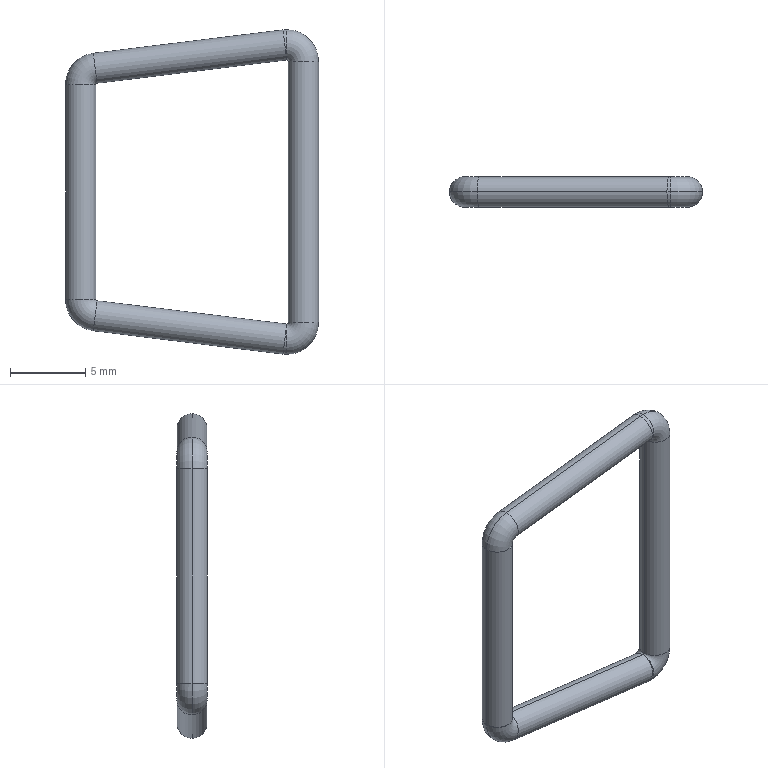Part | SolidWorks | features RefAxis 6, Revolution 4, ICE 3, 3DProfileFeature 2, Extrusion 1 | 1 solid | 24 faces | box 16.763 x 2 x 21.5 mm | volume 200.249 mm3 | torus 12 | cylinder 8 | plane 4 | commonest cylinder face diameters 2 x8
STEP:
#1=CARTESIAN_POINT('',(-7.193,0.,7.107));
#2=VERTEX_POINT('',#1);
#3=CARTESIAN_POINT('',(-6.185,1.,7.107));
#4=VERTEX_POINT('',#3);
#5=CARTESIAN_POINT('',(-6.193,0.,7.107));
#6=DIRECTION('',(0.,0.,-1.));
#7=DIRECTION('',(-1.,0.,0.));
#8=AXIS2_PLACEMENT_3D('',#5,#6,#7);
#9=CIRCLE('',#8,1.);
#10=EDGE_CURVE('',#2,#4,#9,.T.);
#11=ORIENTED_EDGE('',*,*,#10,.F.);
#12=CARTESIAN_POINT('',(-5.349,0.,9.192));
#13=VERTEX_POINT('',#12);
#14=CARTESIAN_POINT('',(-5.093,0.,7.107));
#15=DIRECTION('',(0.,1.,0.));
#16=DIRECTION('',(0.,0.,1.));
#17=AXIS2_PLACEMENT_3D('',#14,#15,#16);
#18=CIRCLE('',#17,2.1);
#19=EDGE_CURVE('',#2,#13,#18,.T.);
#20=ORIENTED_EDGE('',*,*,#19,.T.);
#21=CARTESIAN_POINT('',(-5.105,0.,7.207));
#22=VERTEX_POINT('',#21);
#23=CARTESIAN_POINT('',(-5.227,0.,8.199));
#24=DIRECTION('',(-0.9925,0.,-0.1219));
#25=DIRECTION('',(-0.1219,0.,0.9925));
#26=AXIS2_PLACEMENT_3D('',#23,#24,#25);
#27=CIRCLE('',#26,1.);
#28=EDGE_CURVE('',#13,#22,#27,.T.);
#29=ORIENTED_EDGE('',*,*,#28,.T.);
#30=CARTESIAN_POINT('',(-5.193,0.,7.107));
#31=VERTEX_POINT('',#30);
#32=CARTESIAN_POINT('',(-5.093,0.,7.107));
#33=DIRECTION('',(0.,1.,0.));
#34=DIRECTION('',(0.,0.,1.));
#35=AXIS2_PLACEMENT_3D('',#32,#33,#34);
#36=CIRCLE('',#35,0.1);
#37=EDGE_CURVE('',#31,#22,#36,.T.);
#38=ORIENTED_EDGE('',*,*,#37,.F.);
#39=CARTESIAN_POINT('',(-6.193,0.,7.107));
#40=DIRECTION('',(0.,0.,-1.));
#41=DIRECTION('',(-1.,0.,0.));
#42=AXIS2_PLACEMENT_3D('',#39,#40,#41);
#43=CIRCLE('',#42,1.);
#44=EDGE_CURVE('',#4,#31,#43,.T.);
#45=ORIENTED_EDGE('',*,*,#44,.F.);
#46=EDGE_LOOP('',(#11,#20,#29,#38,#45));
#47=FACE_OUTER_BOUND('',#46,.T.);
#48=CARTESIAN_POINT('',(-5.093,0.,7.107));
#49=DIRECTION('',(0.,1.,0.));
#50=DIRECTION('',(0.,0.,1.));
#51=AXIS2_PLACEMENT_3D('',#48,#49,#50);
#52=TOROIDAL_SURFACE('',#51,1.1,1.);
#53=ADVANCED_FACE('',(#47),#52,.T.);
#54=CARTESIAN_POINT('',(-7.193,0.,-7.107));
#55=VERTEX_POINT('',#54);
#56=CARTESIAN_POINT('',(-6.185,-1.,-7.107));
#57=VERTEX_POINT('',#56);
#58=CARTESIAN_POINT('',(-6.193,0.,-7.107));
#59=DIRECTION('',(0.,0.,1.));
#60=DIRECTION('',(1.,0.,0.));
#61=AXIS2_PLACEMENT_3D('',#58,#59,#60);
#62=CIRCLE('',#61,1.);
#63=EDGE_CURVE('',#55,#57,#62,.T.);
#64=ORIENTED_EDGE('',*,*,#63,.F.);
#65=CARTESIAN_POINT('',(-5.349,0.,-9.192));
#66=VERTEX_POINT('',#65);
#67=CARTESIAN_POINT('',(-5.093,0.,-7.107));
#68=DIRECTION('',(0.,-1.,0.));
#69=DIRECTION('',(0.,0.,-1.));
#70=AXIS2_PLACEMENT_3D('',#67,#68,#69);
#71=CIRCLE('',#70,2.1);
#72=EDGE_CURVE('',#55,#66,#71,.T.);
#73=ORIENTED_EDGE('',*,*,#72,.T.);
#74=CARTESIAN_POINT('',(-5.105,0.,-7.207));
#75=VERTEX_POINT('',#74);
#76=CARTESIAN_POINT('',(-5.227,0.,-8.199));
#77=DIRECTION('',(-0.9925,0.,0.1219));
#78=DIRECTION('',(0.1219,0.,0.9925));
#79=AXIS2_PLACEMENT_3D('',#76,#77,#78);
#80=CIRCLE('',#79,1.);
#81=EDGE_CURVE('',#66,#75,#80,.T.);
#82=ORIENTED_EDGE('',*,*,#81,.T.);
#83=CARTESIAN_POINT('',(-5.193,0.,-7.107));
#84=VERTEX_POINT('',#83);
#85=CARTESIAN_POINT('',(-5.093,0.,-7.107));
#86=DIRECTION('',(0.,-1.,0.));
#87=DIRECTION('',(0.,0.,-1.));
#88=AXIS2_PLACEMENT_3D('',#85,#86,#87);
#89=CIRCLE('',#88,0.1);
#90=EDGE_CURVE('',#84,#75,#89,.T.);
#91=ORIENTED_EDGE('',*,*,#90,.F.);
#92=CARTESIAN_POINT('',(-6.193,0.,-7.107));
#93=DIRECTION('',(0.,0.,1.));
#94=DIRECTION('',(1.,0.,0.));
#95=AXIS2_PLACEMENT_3D('',#92,#93,#94);
#96=CIRCLE('',#95,1.);
#97=EDGE_CURVE('',#57,#84,#96,.T.);
#98=ORIENTED_EDGE('',*,*,#97,.F.);
#99=EDGE_LOOP('',(#64,#73,#82,#91,#98));
#100=FACE_OUTER_BOUND('',#99,.T.);
#101=CARTESIAN_POINT('',(-5.093,0.,-7.107));
#102=DIRECTION('',(0.,-1.,0.));
#103=DIRECTION('',(0.,0.,-1.));
#104=AXIS2_PLACEMENT_3D('',#101,#102,#103);
#105=TOROIDAL_SURFACE('',#104,1.1,1.);
#106=ADVANCED_FACE('',(#100),#105,.T.);
#107=CARTESIAN_POINT('',(7.47,0.,10.75));
#108=VERTEX_POINT('',#107);
#109=CARTESIAN_POINT('',(7.47,0.,8.75));
#110=VERTEX_POINT('',#109);
#111=CARTESIAN_POINT('',(7.47,0.,9.75));
#112=DIRECTION('',(-1.,0.,0.));
#113=DIRECTION('',(0.,0.,1.));
#114=AXIS2_PLACEMENT_3D('',#111,#112,#113);
#115=CIRCLE('',#114,1.);
#116=EDGE_CURVE('',#108,#110,#115,.T.);
#117=ORIENTED_EDGE('',*,*,#116,.F.);
#118=CARTESIAN_POINT('',(9.57,0.,8.65));
#119=VERTEX_POINT('',#118);
#120=CARTESIAN_POINT('',(7.47,0.,8.65));
#121=DIRECTION('',(0.,1.,0.));
#122=DIRECTION('',(0.,0.,1.));
#123=AXIS2_PLACEMENT_3D('',#120,#121,#122);
#124=CIRCLE('',#123,2.1);
#125=EDGE_CURVE('',#108,#119,#124,.T.);
#126=ORIENTED_EDGE('',*,*,#125,.T.);
#127=CARTESIAN_POINT('',(7.57,0.,8.65));
#128=VERTEX_POINT('',#127);
#129=CARTESIAN_POINT('',(8.57,0.,8.65));
#130=DIRECTION('',(0.,0.,1.));
#131=DIRECTION('',(1.,0.,0.));
#132=AXIS2_PLACEMENT_3D('',#129,#130,#131);
#133=CIRCLE('',#132,1.);
#134=EDGE_CURVE('',#119,#128,#133,.T.);
#135=ORIENTED_EDGE('',*,*,#134,.T.);
#136=CARTESIAN_POINT('',(7.47,0.,8.65));
#137=DIRECTION('',(0.,1.,0.));
#138=DIRECTION('',(0.,0.,1.));
#139=AXIS2_PLACEMENT_3D('',#136,#137,#138);
#140=CIRCLE('',#139,0.1);
#141=EDGE_CURVE('',#110,#128,#140,.T.);
#142=ORIENTED_EDGE('',*,*,#141,.F.);
#143=EDGE_LOOP('',(#117,#126,#135,#142));
#144=FACE_OUTER_BOUND('',#143,.T.);
#145=CARTESIAN_POINT('',(7.47,0.,8.65));
#146=DIRECTION('',(0.,1.,0.));
#147=DIRECTION('',(0.,0.,1.));
#148=AXIS2_PLACEMENT_3D('',#145,#146,#147);
#149=TOROIDAL_SURFACE('',#148,1.1,1.);
#150=ADVANCED_FACE('',(#144),#149,.T.);
#151=CARTESIAN_POINT('',(7.47,0.,-10.75));
#152=VERTEX_POINT('',#151);
#153=CARTESIAN_POINT('',(7.47,0.,-8.75));
#154=VERTEX_POINT('',#153);
#155=CARTESIAN_POINT('',(7.47,0.,-9.75));
#156=DIRECTION('',(-1.,0.,0.));
#157=DIRECTION('',(0.,0.,1.));
#158=AXIS2_PLACEMENT_3D('',#155,#156,#157);
#159=CIRCLE('',#158,1.);
#160=EDGE_CURVE('',#152,#154,#159,.T.);
#161=ORIENTED_EDGE('',*,*,#160,.F.);
#162=CARTESIAN_POINT('',(9.57,0.,-8.65));
#163=VERTEX_POINT('',#162);
#164=CARTESIAN_POINT('',(7.47,0.,-8.65));
#165=DIRECTION('',(0.,-1.,0.));
#166=DIRECTION('',(0.,0.,-1.));
#167=AXIS2_PLACEMENT_3D('',#164,#165,#166);
#168=CIRCLE('',#167,2.1);
#169=EDGE_CURVE('',#152,#163,#168,.T.);
#170=ORIENTED_EDGE('',*,*,#169,.T.);
#171=CARTESIAN_POINT('',(7.57,0.,-8.65));
#172=VERTEX_POINT('',#171);
#173=CARTESIAN_POINT('',(8.57,0.,-8.65));
#174=DIRECTION('',(0.,0.,1.));
#175=DIRECTION('',(1.,0.,0.));
#176=AXIS2_PLACEMENT_3D('',#173,#174,#175);
#177=CIRCLE('',#176,1.);
#178=EDGE_CURVE('',#172,#163,#177,.T.);
#179=ORIENTED_EDGE('',*,*,#178,.F.);
#180=CARTESIAN_POINT('',(7.47,0.,-8.65));
#181=DIRECTION('',(0.,-1.,0.));
#182=DIRECTION('',(0.,0.,-1.));
#183=AXIS2_PLACEMENT_3D('',#180,#181,#182);
#184=CIRCLE('',#183,0.1);
#185=EDGE_CURVE('',#154,#172,#184,.T.);
#186=ORIENTED_EDGE('',*,*,#185,.F.);
#187=EDGE_LOOP('',(#161,#170,#179,#186));
#188=FACE_OUTER_BOUND('',#187,.T.);
#189=CARTESIAN_POINT('',(7.47,0.,-8.65));
#190=DIRECTION('',(0.,-1.,0.));
#191=DIRECTION('',(0.,0.,-1.));
#192=AXIS2_PLACEMENT_3D('',#189,#190,#191);
#193=TOROIDAL_SURFACE('',#192,1.1,1.);
#194=ADVANCED_FACE('',(#188),#193,.T.);
#195=CARTESIAN_POINT('',(7.214,0.,-10.734));
#196=VERTEX_POINT('',#195);
#197=CARTESIAN_POINT('',(7.458,0.,-8.749));
#198=VERTEX_POINT('',#197);
#199=CARTESIAN_POINT('',(7.336,0.,-9.742));
#200=DIRECTION('',(-0.9925,0.,0.1219));
#201=DIRECTION('',(0.1219,0.,0.9925));
#202=AXIS2_PLACEMENT_3D('',#199,#200,#201);
#203=CIRCLE('',#202,1.);
#204=EDGE_CURVE('',#196,#198,#203,.T.);
#205=ORIENTED_EDGE('',*,*,#204,.F.);
#206=CARTESIAN_POINT('',(7.47,0.,-8.65));
#207=DIRECTION('',(0.,-1.,0.));
#208=DIRECTION('',(0.,0.,-1.));
#209=AXIS2_PLACEMENT_3D('',#206,#207,#208);
#210=CIRCLE('',#209,2.1);
#211=EDGE_CURVE('',#196,#152,#210,.T.);
#212=ORIENTED_EDGE('',*,*,#211,.T.);
#213=ORIENTED_EDGE('',*,*,#160,.T.);
#214=CARTESIAN_POINT('',(7.47,0.,-8.65));
#215=DIRECTION('',(0.,-1.,0.));
#216=DIRECTION('',(0.,0.,-1.));
#217=AXIS2_PLACEMENT_3D('',#214,#215,#216);
#218=CIRCLE('',#217,0.1);
#219=EDGE_CURVE('',#198,#154,#218,.T.);
#220=ORIENTED_EDGE('',*,*,#219,.F.);
#221=EDGE_LOOP('',(#205,#212,#213,#220));
#222=FACE_OUTER_BOUND('',#221,.T.);
#223=CARTESIAN_POINT('',(7.47,0.,-8.65));
#224=DIRECTION('',(0.,-1.,0.));
#225=DIRECTION('',(0.,0.,-1.));
#226=AXIS2_PLACEMENT_3D('',#223,#224,#225);
#227=TOROIDAL_SURFACE('',#226,1.1,1.);
#228=ADVANCED_FACE('',(#222),#227,.T.);
#229=CARTESIAN_POINT('',(7.214,0.,10.734));
#230=VERTEX_POINT('',#229);
#231=CARTESIAN_POINT('',(7.458,0.,8.749));
#232=VERTEX_POINT('',#231);
#233=CARTESIAN_POINT('',(7.336,0.,9.742));
#234=DIRECTION('',(-0.9925,0.,-0.1219));
#235=DIRECTION('',(-0.1219,0.,0.9925));
#236=AXIS2_PLACEMENT_3D('',#233,#234,#235);
#237=CIRCLE('',#236,1.);
#238=EDGE_CURVE('',#230,#232,#237,.T.);
#239=ORIENTED_EDGE('',*,*,#238,.F.);
#240=CARTESIAN_POINT('',(7.47,0.,8.65));
#241=DIRECTION('',(0.,1.,0.));
#242=DIRECTION('',(0.,0.,1.));
#243=AXIS2_PLACEMENT_3D('',#240,#241,#242);
#244=CIRCLE('',#243,2.1);
#245=EDGE_CURVE('',#230,#108,#244,.T.);
#246=ORIENTED_EDGE('',*,*,#245,.T.);
#247=ORIENTED_EDGE('',*,*,#116,.T.);
#248=CARTESIAN_POINT('',(7.47,0.,8.65));
#249=DIRECTION('',(0.,1.,0.));
#250=DIRECTION('',(0.,0.,1.));
#251=AXIS2_PLACEMENT_3D('',#248,#249,#250);
#252=CIRCLE('',#251,0.1);
#253=EDGE_CURVE('',#232,#110,#252,.T.);
#254=ORIENTED_EDGE('',*,*,#253,.F.);
#255=EDGE_LOOP('',(#239,#246,#247,#254));
#256=FACE_OUTER_BOUND('',#255,.T.);
#257=CARTESIAN_POINT('',(7.47,0.,8.65));
#258=DIRECTION('',(0.,1.,0.));
#259=DIRECTION('',(0.,0.,1.));
#260=AXIS2_PLACEMENT_3D('',#257,#258,#259);
#261=TOROIDAL_SURFACE('',#260,1.1,1.);
#262=ADVANCED_FACE('',(#256),#261,.T.);
#263=CARTESIAN_POINT('',(-5.177,0.,7.107));
#264=VERTEX_POINT('',#263);
#265=CARTESIAN_POINT('',(-6.177,0.,7.107));
#266=DIRECTION('',(0.,0.,1.));
#267=DIRECTION('',(1.,0.,0.));
#268=AXIS2_PLACEMENT_3D('',#265,#266,#267);
#269=CIRCLE('',#268,1.);
#270=EDGE_CURVE('',#264,#4,#269,.T.);
#271=ORIENTED_EDGE('',*,*,#270,.F.);
#272=CARTESIAN_POINT('',(-5.177,0.,-7.107));
#273=VERTEX_POINT('',#272);
#274=CARTESIAN_POINT('',(-5.177,0.,7.107));
#275=DIRECTION('',(0.,0.,-1.));
#276=VECTOR('',#275,1000.);
#277=LINE('',#274,#276);
#278=EDGE_CURVE('',#264,#273,#277,.T.);
#279=ORIENTED_EDGE('',*,*,#278,.T.);
#280=CARTESIAN_POINT('',(-6.185,1.,-7.107));
#281=VERTEX_POINT('',#280);
#282=CARTESIAN_POINT('',(-6.177,0.,-7.107));
#283=DIRECTION('',(0.,0.,1.));
#284=DIRECTION('',(1.,0.,0.));
#285=AXIS2_PLACEMENT_3D('',#282,#283,#284);
#286=CIRCLE('',#285,1.);
#287=EDGE_CURVE('',#273,#281,#286,.T.);
#288=ORIENTED_EDGE('',*,*,#287,.T.);
#289=CARTESIAN_POINT('',(-7.177,0.,-7.107));
#290=VERTEX_POINT('',#289);
#291=CARTESIAN_POINT('',(-6.177,0.,-7.107));
#292=DIRECTION('',(0.,0.,1.));
#293=DIRECTION('',(1.,0.,0.));
#294=AXIS2_PLACEMENT_3D('',#291,#292,#293);
#295=CIRCLE('',#294,1.);
#296=EDGE_CURVE('',#281,#290,#295,.T.);
#297=ORIENTED_EDGE('',*,*,#296,.T.);
#298=CARTESIAN_POINT('',(-7.177,0.,7.107));
#299=VERTEX_POINT('',#298);
#300=CARTESIAN_POINT('',(-7.177,0.,7.107));
#301=DIRECTION('',(0.,0.,-1.));
#302=VECTOR('',#301,1000.);
#303=LINE('',#300,#302);
#304=EDGE_CURVE('',#299,#290,#303,.T.);
#305=ORIENTED_EDGE('',*,*,#304,.F.);
#306=CARTESIAN_POINT('',(-6.177,0.,7.107));
#307=DIRECTION('',(0.,0.,1.));
#308=DIRECTION('',(1.,0.,0.));
#309=AXIS2_PLACEMENT_3D('',#306,#307,#308);
#310=CIRCLE('',#309,1.);
#311=EDGE_CURVE('',#4,#299,#310,.T.);
#312=ORIENTED_EDGE('',*,*,#311,.F.);
#313=EDGE_LOOP('',(#271,#279,#288,#297,#305,#312));
#314=FACE_OUTER_BOUND('',#313,.T.);
#315=CARTESIAN_POINT('',(-6.177,0.,7.107));
#316=DIRECTION('',(0.,0.,-1.));
#317=DIRECTION('',(-1.,0.,0.));
#318=AXIS2_PLACEMENT_3D('',#315,#316,#317);
#319=CYLINDRICAL_SURFACE('',#318,1.);
#320=ADVANCED_FACE('',(#314),#319,.T.);
#321=ORIENTED_EDGE('',*,*,#28,.F.);
#322=CARTESIAN_POINT('',(-5.349,0.,9.192));
#323=DIRECTION('',(0.9925,0.,0.1219));
#324=VECTOR('',#323,1000.);
#325=LINE('',#322,#324);
#326=EDGE_CURVE('',#13,#230,#325,.T.);
#327=ORIENTED_EDGE('',*,*,#326,.T.);
#328=ORIENTED_EDGE('',*,*,#238,.T.);
#329=CARTESIAN_POINT('',(-5.105,0.,7.207));
#330=DIRECTION('',(0.9925,0.,0.1219));
#331=VECTOR('',#330,1000.);
#332=LINE('',#329,#331);
#333=EDGE_CURVE('',#22,#232,#332,.T.);
#334=ORIENTED_EDGE('',*,*,#333,.F.);
#335=EDGE_LOOP('',(#321,#327,#328,#334));
#336=FACE_OUTER_BOUND('',#335,.T.);
#337=CARTESIAN_POINT('',(-5.227,0.,8.199));
#338=DIRECTION('',(0.9925,0.,0.1219));
#339=DIRECTION('',(0.1219,0.,-0.9925));
#340=AXIS2_PLACEMENT_3D('',#337,#338,#339);
#341=CYLINDRICAL_SURFACE('',#340,1.);
#342=ADVANCED_FACE('',(#336),#341,.T.);
#343=CARTESIAN_POINT('',(-5.227,0.,-8.199));
#344=DIRECTION('',(-0.9925,0.,0.1219));
#345=DIRECTION('',(0.1219,0.,0.9925));
#346=AXIS2_PLACEMENT_3D('',#343,#344,#345);
#347=CIRCLE('',#346,1.);
#348=EDGE_CURVE('',#75,#66,#347,.T.);
#349=ORIENTED_EDGE('',*,*,#348,.F.);
#350=CARTESIAN_POINT('',(-5.105,0.,-7.207));
#351=DIRECTION('',(0.9925,0.,-0.1219));
#352=VECTOR('',#351,1000.);
#353=LINE('',#350,#352);
#354=EDGE_CURVE('',#75,#198,#353,.T.);
#355=ORIENTED_EDGE('',*,*,#354,.T.);
#356=CARTESIAN_POINT('',(7.336,0.,-9.742));
#357=DIRECTION('',(-0.9925,0.,0.1219));
#358=DIRECTION('',(0.1219,0.,0.9925));
#359=AXIS2_PLACEMENT_3D('',#356,#357,#358);
#360=CIRCLE('',#359,1.);
#361=EDGE_CURVE('',#198,#196,#360,.T.);
#362=ORIENTED_EDGE('',*,*,#361,.T.);
#363=CARTESIAN_POINT('',(-5.349,0.,-9.192));
#364=DIRECTION('',(0.9925,0.,-0.1219));
#365=VECTOR('',#364,1000.);
#366=LINE('',#363,#365);
#367=EDGE_CURVE('',#66,#196,#366,.T.);
#368=ORIENTED_EDGE('',*,*,#367,.F.);
#369=EDGE_LOOP('',(#349,#355,#362,#368));
#370=FACE_OUTER_BOUND('',#369,.T.);
#371=CARTESIAN_POINT('',(-5.227,0.,-8.199));
#372=DIRECTION('',(0.9925,0.,-0.1219));
#373=DIRECTION('',(-0.1219,0.,-0.9925));
#374=AXIS2_PLACEMENT_3D('',#371,#372,#373);
#375=CYLINDRICAL_SURFACE('',#374,1.);
#376=ADVANCED_FACE('',(#370),#375,.T.);
#377=ORIENTED_EDGE('',*,*,#245,.F.);
#378=CARTESIAN_POINT('',(7.336,0.,9.742));
#379=DIRECTION('',(-0.9925,0.,-0.1219));
#380=DIRECTION('',(-0.1219,0.,0.9925));
#381=AXIS2_PLACEMENT_3D('',#378,#379,#380);
#382=CIRCLE('',#381,1.);
#383=EDGE_CURVE('',#232,#230,#382,.T.);
#384=ORIENTED_EDGE('',*,*,#383,.F.);
#385=ORIENTED_EDGE('',*,*,#253,.T.);
#386=CARTESIAN_POINT('',(7.47,0.,9.75));
#387=DIRECTION('',(-1.,0.,0.));
#388=DIRECTION('',(0.,0.,1.));
#389=AXIS2_PLACEMENT_3D('',#386,#387,#388);
#390=CIRCLE('',#389,1.);
#391=EDGE_CURVE('',#110,#108,#390,.T.);
#392=ORIENTED_EDGE('',*,*,#391,.T.);
#393=EDGE_LOOP('',(#377,#384,#385,#392));
#394=FACE_OUTER_BOUND('',#393,.T.);
#395=CARTESIAN_POINT('',(7.47,0.,8.65));
#396=DIRECTION('',(0.,1.,0.));
#397=DIRECTION('',(0.,0.,1.));
#398=AXIS2_PLACEMENT_3D('',#395,#396,#397);
#399=TOROIDAL_SURFACE('',#398,1.1,1.);
#400=ADVANCED_FACE('',(#394),#399,.T.);
#401=ORIENTED_EDGE('',*,*,#211,.F.);
#402=ORIENTED_EDGE('',*,*,#361,.F.);
#403=ORIENTED_EDGE('',*,*,#219,.T.);
#404=CARTESIAN_POINT('',(7.47,0.,-9.75));
#405=DIRECTION('',(-1.,0.,0.));
#406=DIRECTION('',(0.,0.,1.));
#407=AXIS2_PLACEMENT_3D('',#404,#405,#406);
#408=CIRCLE('',#407,1.);
#409=EDGE_CURVE('',#154,#152,#408,.T.);
#410=ORIENTED_EDGE('',*,*,#409,.T.);
#411=EDGE_LOOP('',(#401,#402,#403,#410));
#412=FACE_OUTER_BOUND('',#411,.T.);
#413=CARTESIAN_POINT('',(7.47,0.,-8.65));
#414=DIRECTION('',(0.,-1.,0.));
#415=DIRECTION('',(0.,0.,-1.));
#416=AXIS2_PLACEMENT_3D('',#413,#414,#415);
#417=TOROIDAL_SURFACE('',#416,1.1,1.);
#418=ADVANCED_FACE('',(#412),#417,.T.);
#419=ORIENTED_EDGE('',*,*,#134,.F.);
#420=CARTESIAN_POINT('',(9.57,0.,8.65));
#421=DIRECTION('',(0.,0.,-1.));
#422=VECTOR('',#421,1000.);
#423=LINE('',#420,#422);
#424=EDGE_CURVE('',#119,#163,#423,.T.);
#425=ORIENTED_EDGE('',*,*,#424,.T.);
#426=CARTESIAN_POINT('',(8.57,0.,-8.65));
#427=DIRECTION('',(0.,0.,1.));
#428=DIRECTION('',(1.,0.,0.));
#429=AXIS2_PLACEMENT_3D('',#426,#427,#428);
#430=CIRCLE('',#429,1.);
#431=EDGE_CURVE('',#163,#172,#430,.T.);
#432=ORIENTED_EDGE('',*,*,#431,.T.);
#433=CARTESIAN_POINT('',(7.57,0.,8.65));
#434=DIRECTION('',(0.,0.,-1.));
#435=VECTOR('',#434,1000.);
#436=LINE('',#433,#435);
#437=EDGE_CURVE('',#128,#172,#436,.T.);
#438=ORIENTED_EDGE('',*,*,#437,.F.);
#439=EDGE_LOOP('',(#419,#425,#432,#438));
#440=FACE_OUTER_BOUND('',#439,.T.);
#441=CARTESIAN_POINT('',(8.57,0.,8.65));
#442=DIRECTION('',(0.,0.,-1.));
#443=DIRECTION('',(-1.,0.,0.));
#444=AXIS2_PLACEMENT_3D('',#441,#442,#443);
#445=CYLINDRICAL_SURFACE('',#444,1.);
#446=ADVANCED_FACE('',(#440),#445,.T.);
#447=CARTESIAN_POINT('',(-6.185,-1.,7.107));
#448=VERTEX_POINT('',#447);
#449=CARTESIAN_POINT('',(-6.193,0.,7.107));
#450=DIRECTION('',(0.,0.,-1.));
#451=DIRECTION('',(-1.,0.,0.));
#452=AXIS2_PLACEMENT_3D('',#449,#450,#451);
#453=CIRCLE('',#452,1.);
#454=EDGE_CURVE('',#448,#2,#453,.T.);
#455=ORIENTED_EDGE('',*,*,#454,.T.);
#456=ORIENTED_EDGE('',*,*,#10,.T.);
#457=ORIENTED_EDGE('',*,*,#311,.T.);
#458=CARTESIAN_POINT('',(-6.177,0.,7.107));
#459=DIRECTION('',(0.,0.,1.));
#460=DIRECTION('',(1.,0.,0.));
#461=AXIS2_PLACEMENT_3D('',#458,#459,#460);
#462=CIRCLE('',#461,1.);
#463=EDGE_CURVE('',#299,#448,#462,.T.);
#464=ORIENTED_EDGE('',*,*,#463,.T.);
#465=EDGE_LOOP('',(#455,#456,#457,#464));
#466=FACE_OUTER_BOUND('',#465,.T.);
#467=CARTESIAN_POINT('',(-6.193,0.,7.107));
#468=DIRECTION('',(0.,0.,-1.));
#469=DIRECTION('',(-1.,0.,0.));
#470=AXIS2_PLACEMENT_3D('',#467,#468,#469);
#471=PLANE('',#470);
#472=ADVANCED_FACE('',(#466),#471,.T.);
#473=ORIENTED_EDGE('',*,*,#424,.F.);
#474=CARTESIAN_POINT('',(8.57,0.,8.65));
#475=DIRECTION('',(0.,0.,1.));
#476=DIRECTION('',(1.,0.,0.));
#477=AXIS2_PLACEMENT_3D('',#474,#475,#476);
#478=CIRCLE('',#477,1.);
#479=EDGE_CURVE('',#128,#119,#478,.T.);
#480=ORIENTED_EDGE('',*,*,#479,.F.);
#481=ORIENTED_EDGE('',*,*,#437,.T.);
#482=ORIENTED_EDGE('',*,*,#178,.T.);
#483=EDGE_LOOP('',(#473,#480,#481,#482));
#484=FACE_OUTER_BOUND('',#483,.T.);
#485=CARTESIAN_POINT('',(8.57,0.,8.65));
#486=DIRECTION('',(0.,0.,-1.));
#487=DIRECTION('',(-1.,0.,0.));
#488=AXIS2_PLACEMENT_3D('',#485,#486,#487);
#489=CYLINDRICAL_SURFACE('',#488,1.);
#490=ADVANCED_FACE('',(#484),#489,.T.);
#491=ORIENTED_EDGE('',*,*,#169,.F.);
#492=ORIENTED_EDGE('',*,*,#409,.F.);
#493=ORIENTED_EDGE('',*,*,#185,.T.);
#494=ORIENTED_EDGE('',*,*,#431,.F.);
#495=EDGE_LOOP('',(#491,#492,#493,#494));
#496=FACE_OUTER_BOUND('',#495,.T.);
#497=CARTESIAN_POINT('',(7.47,0.,-8.65));
#498=DIRECTION('',(0.,-1.,0.));
#499=DIRECTION('',(0.,0.,-1.));
#500=AXIS2_PLACEMENT_3D('',#497,#498,#499);
#501=TOROIDAL_SURFACE('',#500,1.1,1.);
#502=ADVANCED_FACE('',(#496),#501,.T.);
#503=ORIENTED_EDGE('',*,*,#125,.F.);
#504=ORIENTED_EDGE('',*,*,#391,.F.);
#505=ORIENTED_EDGE('',*,*,#141,.T.);
#506=ORIENTED_EDGE('',*,*,#479,.T.);
#507=EDGE_LOOP('',(#503,#504,#505,#506));
#508=FACE_OUTER_BOUND('',#507,.T.);
#509=CARTESIAN_POINT('',(7.47,0.,8.65));
#510=DIRECTION('',(0.,1.,0.));
#511=DIRECTION('',(0.,0.,1.));
#512=AXIS2_PLACEMENT_3D('',#509,#510,#511);
#513=TOROIDAL_SURFACE('',#512,1.1,1.);
#514=ADVANCED_FACE('',(#508),#513,.T.);
#515=ORIENTED_EDGE('',*,*,#354,.F.);
#516=ORIENTED_EDGE('',*,*,#81,.F.);
#517=ORIENTED_EDGE('',*,*,#367,.T.);
#518=ORIENTED_EDGE('',*,*,#204,.T.);
#519=EDGE_LOOP('',(#515,#516,#517,#518));
#520=FACE_OUTER_BOUND('',#519,.T.);
#521=CARTESIAN_POINT('',(-5.227,0.,-8.199));
#522=DIRECTION('',(0.9925,0.,-0.1219));
#523=DIRECTION('',(-0.1219,0.,-0.9925));
#524=AXIS2_PLACEMENT_3D('',#521,#522,#523);
#525=CYLINDRICAL_SURFACE('',#524,1.);
#526=ADVANCED_FACE('',(#520),#525,.T.);
#527=ORIENTED_EDGE('',*,*,#326,.F.);
#528=CARTESIAN_POINT('',(-5.227,0.,8.199));
#529=DIRECTION('',(-0.9925,0.,-0.1219));
#530=DIRECTION('',(-0.1219,0.,0.9925));
#531=AXIS2_PLACEMENT_3D('',#528,#529,#530);
#532=CIRCLE('',#531,1.);
#533=EDGE_CURVE('',#22,#13,#532,.T.);
#534=ORIENTED_EDGE('',*,*,#533,.F.);
#535=ORIENTED_EDGE('',*,*,#333,.T.);
#536=ORIENTED_EDGE('',*,*,#383,.T.);
#537=EDGE_LOOP('',(#527,#534,#535,#536));
#538=FACE_OUTER_BOUND('',#537,.T.);
#539=CARTESIAN_POINT('',(-5.227,0.,8.199));
#540=DIRECTION('',(0.9925,0.,0.1219));
#541=DIRECTION('',(0.1219,0.,-0.9925));
#542=AXIS2_PLACEMENT_3D('',#539,#540,#541);
#543=CYLINDRICAL_SURFACE('',#542,1.);
#544=ADVANCED_FACE('',(#538),#543,.T.);
#545=ORIENTED_EDGE('',*,*,#72,.F.);
#546=CARTESIAN_POINT('',(-6.193,0.,-7.107));
#547=DIRECTION('',(0.,0.,1.));
#548=DIRECTION('',(1.,0.,0.));
#549=AXIS2_PLACEMENT_3D('',#546,#547,#548);
#550=CIRCLE('',#549,1.);
#551=EDGE_CURVE('',#281,#55,#550,.T.);
#552=ORIENTED_EDGE('',*,*,#551,.F.);
#553=CARTESIAN_POINT('',(-6.193,0.,-7.107));
#554=DIRECTION('',(0.,0.,1.));
#555=DIRECTION('',(1.,0.,0.));
#556=AXIS2_PLACEMENT_3D('',#553,#554,#555);
#557=CIRCLE('',#556,1.);
#558=EDGE_CURVE('',#84,#281,#557,.T.);
#559=ORIENTED_EDGE('',*,*,#558,.F.);
#560=ORIENTED_EDGE('',*,*,#90,.T.);
#561=ORIENTED_EDGE('',*,*,#348,.T.);
#562=EDGE_LOOP('',(#545,#552,#559,#560,#561));
#563=FACE_OUTER_BOUND('',#562,.T.);
#564=CARTESIAN_POINT('',(-5.093,0.,-7.107));
#565=DIRECTION('',(0.,-1.,0.));
#566=DIRECTION('',(0.,0.,-1.));
#567=AXIS2_PLACEMENT_3D('',#564,#565,#566);
#568=TOROIDAL_SURFACE('',#567,1.1,1.);
#569=ADVANCED_FACE('',(#563),#568,.T.);
#570=ORIENTED_EDGE('',*,*,#296,.F.);
#571=ORIENTED_EDGE('',*,*,#551,.T.);
#572=ORIENTED_EDGE('',*,*,#63,.T.);
#573=CARTESIAN_POINT('',(-6.177,0.,-7.107));
#574=DIRECTION('',(0.,0.,1.));
#575=DIRECTION('',(1.,0.,0.));
#576=AXIS2_PLACEMENT_3D('',#573,#574,#575);
#577=CIRCLE('',#576,1.);
#578=EDGE_CURVE('',#290,#57,#577,.T.);
#579=ORIENTED_EDGE('',*,*,#578,.F.);
#580=EDGE_LOOP('',(#570,#571,#572,#579));
#581=FACE_OUTER_BOUND('',#580,.T.);
#582=CARTESIAN_POINT('',(-6.193,0.,-7.107));
#583=DIRECTION('',(0.,0.,1.));
#584=DIRECTION('',(1.,0.,0.));
#585=AXIS2_PLACEMENT_3D('',#582,#583,#584);
#586=PLANE('',#585);
#587=ADVANCED_FACE('',(#581),#586,.T.);
#588=ORIENTED_EDGE('',*,*,#19,.F.);
#589=ORIENTED_EDGE('',*,*,#454,.F.);
#590=CARTESIAN_POINT('',(-6.193,0.,7.107));
#591=DIRECTION('',(0.,0.,-1.));
#592=DIRECTION('',(-1.,0.,0.));
#593=AXIS2_PLACEMENT_3D('',#590,#591,#592);
#594=CIRCLE('',#593,1.);
#595=EDGE_CURVE('',#31,#448,#594,.T.);
#596=ORIENTED_EDGE('',*,*,#595,.F.);
#597=ORIENTED_EDGE('',*,*,#37,.T.);
#598=ORIENTED_EDGE('',*,*,#533,.T.);
#599=EDGE_LOOP('',(#588,#589,#596,#597,#598));
#600=FACE_OUTER_BOUND('',#599,.T.);
#601=CARTESIAN_POINT('',(-5.093,0.,7.107));
#602=DIRECTION('',(0.,1.,0.));
#603=DIRECTION('',(0.,0.,1.));
#604=AXIS2_PLACEMENT_3D('',#601,#602,#603);
#605=TOROIDAL_SURFACE('',#604,1.1,1.);
#606=ADVANCED_FACE('',(#600),#605,.T.);
#607=CARTESIAN_POINT('',(-6.177,0.,-7.107));
#608=DIRECTION('',(0.,0.,1.));
#609=DIRECTION('',(1.,0.,0.));
#610=AXIS2_PLACEMENT_3D('',#607,#608,#609);
#611=CIRCLE('',#610,1.);
#612=EDGE_CURVE('',#57,#273,#611,.T.);
#613=ORIENTED_EDGE('',*,*,#612,.F.);
#614=ORIENTED_EDGE('',*,*,#97,.T.);
#615=ORIENTED_EDGE('',*,*,#558,.T.);
#616=ORIENTED_EDGE('',*,*,#287,.F.);
#617=EDGE_LOOP('',(#613,#614,#615,#616));
#618=FACE_OUTER_BOUND('',#617,.T.);
#619=CARTESIAN_POINT('',(-6.177,0.,-7.107));
#620=DIRECTION('',(0.,0.,1.));
#621=DIRECTION('',(1.,0.,0.));
#622=AXIS2_PLACEMENT_3D('',#619,#620,#621);
#623=PLANE('',#622);
#624=ADVANCED_FACE('',(#618),#623,.F.);
#625=ORIENTED_EDGE('',*,*,#278,.F.);
#626=CARTESIAN_POINT('',(-6.177,0.,7.107));
#627=DIRECTION('',(0.,0.,1.));
#628=DIRECTION('',(1.,0.,0.));
#629=AXIS2_PLACEMENT_3D('',#626,#627,#628);
#630=CIRCLE('',#629,1.);
#631=EDGE_CURVE('',#448,#264,#630,.T.);
#632=ORIENTED_EDGE('',*,*,#631,.F.);
#633=ORIENTED_EDGE('',*,*,#463,.F.);
#634=ORIENTED_EDGE('',*,*,#304,.T.);
#635=ORIENTED_EDGE('',*,*,#578,.T.);
#636=ORIENTED_EDGE('',*,*,#612,.T.);
#637=EDGE_LOOP('',(#625,#632,#633,#634,#635,#636));
#638=FACE_OUTER_BOUND('',#637,.T.);
#639=CARTESIAN_POINT('',(-6.177,0.,7.107));
#640=DIRECTION('',(0.,0.,-1.));
#641=DIRECTION('',(-1.,0.,0.));
#642=AXIS2_PLACEMENT_3D('',#639,#640,#641);
#643=CYLINDRICAL_SURFACE('',#642,1.);
#644=ADVANCED_FACE('',(#638),#643,.T.);
#645=ORIENTED_EDGE('',*,*,#631,.T.);
#646=ORIENTED_EDGE('',*,*,#270,.T.);
#647=ORIENTED_EDGE('',*,*,#44,.T.);
#648=ORIENTED_EDGE('',*,*,#595,.T.);
#649=EDGE_LOOP('',(#645,#646,#647,#648));
#650=FACE_OUTER_BOUND('',#649,.T.);
#651=CARTESIAN_POINT('',(-6.177,0.,7.107));
#652=DIRECTION('',(0.,0.,1.));
#653=DIRECTION('',(1.,0.,0.));
#654=AXIS2_PLACEMENT_3D('',#651,#652,#653);
#655=PLANE('',#654);
#656=ADVANCED_FACE('',(#650),#655,.T.);
#657=CLOSED_SHELL('',(#53,#106,#150,#194,#228,#262,#320,#342,#376,#400,#418,#446,#472,#490,#502,#514,#526,#544,#569,#587,#606,#624,#644,#656));
#658=MANIFOLD_SOLID_BREP('',#657);
#659=CARTESIAN_POINT('',(0.,0.,0.));
#660=DIRECTION('',(0.,0.,1.));
#661=DIRECTION('',(1.,0.,0.));
#662=AXIS2_PLACEMENT_3D('',#659,#660,#661);
#663=(LENGTH_UNIT()NAMED_UNIT(*)SI_UNIT(.MILLI.,.METRE.));
#664=UNCERTAINTY_MEASURE_WITH_UNIT(LENGTH_MEASURE(0.00001),#663,'','');
#665=(NAMED_UNIT(*)PLANE_ANGLE_UNIT()SI_UNIT($,.RADIAN.));
#666=(NAMED_UNIT(*)SI_UNIT($,.STERADIAN.)SOLID_ANGLE_UNIT());
#667=(GEOMETRIC_REPRESENTATION_CONTEXT(3)GLOBAL_UNCERTAINTY_ASSIGNED_CONTEXT((#664))GLOBAL_UNIT_ASSIGNED_CONTEXT((#663,#665,#666))REPRESENTATION_CONTEXT('',''));
#668=ADVANCED_BREP_SHAPE_REPRESENTATION('',(#658,#662),#667);